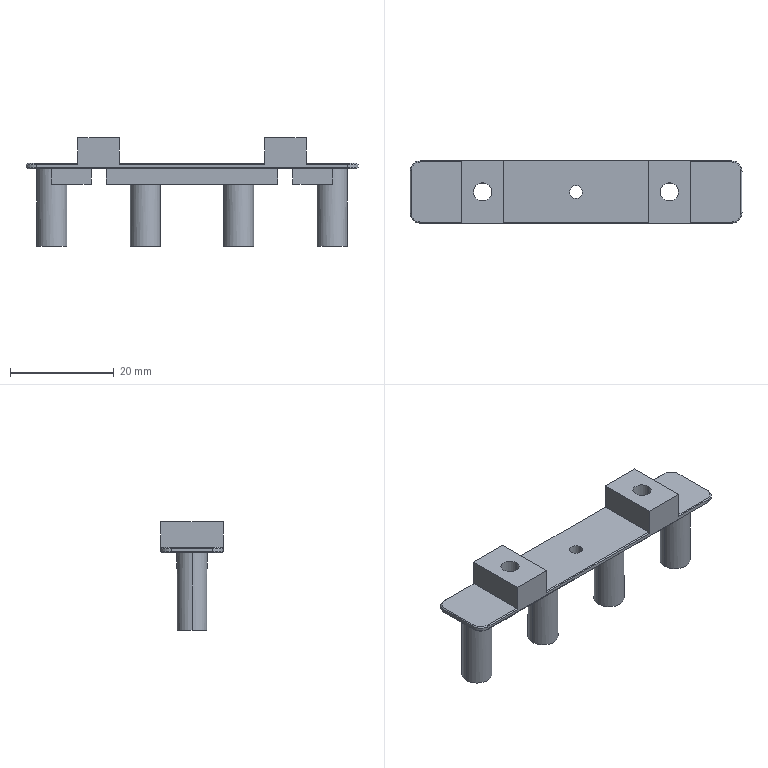NC program | NX | posted with a generic post | part box 64 x 12 x 21 mm
Lines 928 to 2253 of 2253:
(FLOOR_WALL_1_COPY_COPY , TOOL : D6)
N1848 T12 M6
N1850 G54
N1852 G17 G0 G90 X21.496 Y-7.4 S9500 M3
N1854 G43 Z30. H12
N1856 Z-10.5
N1858 G94 G1 Z-12. F1500.
N1860 Y-3.497
N1862 G3 X21.518 Y-2.897 R0.6
N1864 G1 X14.482
N1866 G3 X15.083 Y-1.199 R6.2
N1868 G1 X20.917
N1870 G2 X20.82 Y0.5 R6.2
N1872 G1 X15.18
N1874 G3 X14.797 Y2.198 R6.2
N1876 G1 X21.203
N1878 G2 X22.178 Y3.897 R6.2
N1880 G1 X13.822
N1882 G3 X11.67 Y5.595 R6.2
N1884 G1 X24.33
N1886 Z-10.5
N1888 G0 Z30.
N1890 X25.8 Y-7.302
N1892 Z-10.5
N1894 G1 Z-12.
N1896 X25.541 Y-6.048
N1898 G3 X25.143 Y-5.6 R0.6
N1900 G2 X25.143 Y5.6 R5.9
N1902 G3 X25.541 Y6.048 R0.6
N1904 G1 X25.8 Y7.302
N1906 Z-10.5
N1908 G0 X10.2
N1910 G1 Z-12.
N1912 X10.459 Y6.048
N1914 G3 X10.857 Y5.6 R0.6
N1916 G2 X10.857 Y-5.6 R5.9
N1918 G3 X10.459 Y-6.048 R0.6
N1920 G1 X10.2 Y-7.302
N1922 Z-10.5
N1924 G0 Z30.
N1926 X3.496 Y-7.4
N1928 Z-10.5
N1930 G1 Z-12.
N1932 Y-3.497
N1934 G3 X3.518 Y-2.897 R0.6
N1936 G1 X-3.518
N1938 G3 X-2.917 Y-1.199 R6.2
N1940 G1 X2.917
N1942 G2 X2.82 Y0.5 R6.2
N1944 G1 X-2.82
N1946 G3 X-3.203 Y2.198 R6.2
N1948 G1 X3.203
N1950 G2 X4.178 Y3.897 R6.2
N1952 G1 X-4.178
N1954 G3 X-6.33 Y5.595 R6.2
N1956 G1 X6.33
N1958 Z-10.5
N1960 G0 Z30.
N1962 X7.8 Y-7.302
N1964 Z-10.5
N1966 G1 Z-12.
N1968 X7.541 Y-6.048
N1970 G3 X7.143 Y-5.6 R0.6
N1972 G2 X7.143 Y5.6 R5.9
N1974 G3 X7.541 Y6.048 R0.6
N1976 G1 X7.8 Y7.302
N1978 Z-10.5
N1980 G0 X-7.8
N1982 G1 Z-12.
N1984 X-7.541 Y6.048
N1986 G3 X-7.143 Y5.6 R0.6
N1988 G2 X-7.143 Y-5.6 R5.9
N1990 G3 X-7.541 Y-6.048 R0.6
N1992 G1 X-7.8 Y-7.302
N1994 Z-10.5
N1996 G0 Z30.
N1998 X-14.504 Y-7.4
N2000 Z-10.5
N2002 G1 Z-12.
N2004 Y-3.497
N2006 G3 X-14.482 Y-2.897 R0.6
N2008 G1 X-21.518
N2010 G3 X-20.917 Y-1.199 R6.2
N2012 G1 X-15.083
N2014 G2 X-15.18 Y0.5 R6.2
N2016 G1 X-20.82
N2018 G3 X-21.203 Y2.198 R6.2
N2020 G1 X-14.797
N2022 G2 X-13.822 Y3.897 R6.2
N2024 G1 X-22.178
N2026 G3 X-24.33 Y5.595 R6.2
N2028 G1 X-11.67
N2030 Z-10.5
N2032 G0 Z30.
N2034 X-10.2 Y-7.302
N2036 Z-10.5
N2038 G1 Z-12.
N2040 X-10.459 Y-6.048
N2042 G3 X-10.857 Y-5.6 R0.6
N2044 G2 X-10.857 Y5.6 R5.9
N2046 G3 X-10.459 Y6.048 R0.6
N2048 G1 X-10.2 Y7.302
N2050 Z-10.5
N2052 G0 X-25.8
N2054 G1 Z-12.
N2056 X-25.541 Y6.048
N2058 G3 X-25.143 Y5.6 R0.6
N2060 G2 X-25.143 Y-5.6 R5.9
N2062 G3 X-25.541 Y-6.048 R0.6
N2064 G1 X-25.8 Y-7.302
N2066 Z-10.5
N2068 G0 Z30.
N2070 X35.548 Y-6.939
N2072 Z-13.5
N2074 G1 Z-15.
N2076 X35.011 Y-6.009
N2078 G3 X34.492 Y-5.709 R0.6
N2080 G1 X29.418
N2082 G3 X32.164 Y-3.432 R6.2
N2084 G1 X34.8
N2086 Y-1.154
N2088 X33.092
N2090 G3 X33.097 Y1.123 R6.2
N2092 G1 X34.8
N2094 Y3.4
N2096 X32.185
N2098 G3 X29.492 Y5.677 R6.2
N2100 G1 X34.508
N2102 G2 X35.027 Y5.377 R0.6
N2104 G1 X36.3 Y3.173
N2106 Z-13.5
N2108 G0 Z30.
N2110 X-29.057 Y-10.3
N2112 Z-13.5
N2114 G1 Z-15.
N2116 Y-6.188
N2118 G3 X-29.418 Y-5.709 R0.6
N2120 G1 X-34.492
N2122 X-34.601 Y-5.495
N2124 X-34.8 Y-4.236
N2126 Y-3.432
N2128 X-32.164
N2130 G2 X-33.092 Y-1.154 R6.2
N2132 G1 X-34.8
N2134 Y1.123
N2136 X-33.097
N2138 G2 X-32.185 Y3.4 R6.2
N2140 G1 X-34.8
N2142 Y4.236
N2144 X-34.601 Y5.495
N2146 X-34.508 Y5.677
N2148 X-29.492
N2150 Z-13.5
N2152 G0 Z30.
N2154 X34.253 Y8.625
N2156 Z-13.5
N2158 G1 Z-15.
N2160 X33.283 Y7.654
N2162 G3 X32.763 Y7.954 R0.6
N2164 G1 X-32.763
N2166 G3 X-33.283 Y7.654 R0.6
N2168 G1 X-31.058 Y4.716
N2170 G3 X-30.462 Y4.778 R0.6
N2172 G2 X-27. Y5.9 R5.9
N2174 G1 X27.
N2176 G2 X32.9 Y0. R5.9
N2178 X27. Y-5.9 R5.9
N2180 G1 X-27.
N2182 G2 X-30.462 Y4.778 R5.9
N2184 G3 X-30.217 Y5.326 R0.6
N2186 G1 X-30.382 Y6.918
N2188 Z-13.5
N2190 G0 Z30.
N2192 X18.11 Y0.224
N2194 Z-13.4
N2196 G1 X18. Y0.28 Z-13.433
N2198 X17.775 Y0.166 Z-13.501
N2200 X17.72 Y0. Z-13.548
N2202 X17.777 Y-0.113 Z-13.582
N2204 X17.814 Y-0.186 Z-13.604
N2206 X18. Y-0.28 Z-13.659
N2208 X18.113 Y-0.223 Z-13.693
N2210 X18.225 Y-0.166 Z-13.727
N2212 X18.28 Y0. Z-13.774
N2214 X18.223 Y0.113 Z-13.808
N2216 X18.186 Y0.186 Z-13.83
N2218 X18. Y0.28 Z-13.886
N2220 X17.775 Y0.166 Z-13.953
N2222 X17.72 Y0. Z-14.
N2224 X17.777 Y-0.113 Z-14.034
N2226 X17.814 Y-0.186 Z-14.056
N2228 X18. Y-0.28 Z-14.112
N2230 X18.113 Y-0.223 Z-14.146
N2232 X18.225 Y-0.166 Z-14.18
N2234 X18.28 Y0. Z-14.227
N2236 X18.223 Y0.113 Z-14.26
N2238 X18.186 Y0.186 Z-14.282
N2240 X18. Y0.28 Z-14.338
N2242 X17.775 Y0.166 Z-14.406
N2244 X17.72 Y0. Z-14.453
N2246 X17.777 Y-0.113 Z-14.487
N2248 X17.814 Y-0.186 Z-14.509
N2250 X18. Y-0.28 Z-14.564
N2252 X18.113 Y-0.223 Z-14.598
N2254 X18.225 Y-0.166 Z-14.632
N2256 X18.28 Y0. Z-14.679
N2258 X18.223 Y0.113 Z-14.713
N2260 X18.186 Y0.186 Z-14.735
N2262 X18. Y0.28 Z-14.791
N2264 X17.775 Y0.166 Z-14.858
N2266 X17.72 Y0. Z-14.905
N2268 X17.777 Y-0.113 Z-14.939
N2270 X17.814 Y-0.186 Z-14.961
N2272 X17.944 Y-0.252 Z-15.
N2274 X18. Y-0.28
N2276 X18.113 Y-0.223
N2278 G3 X18.113 Y0.223 R0.25
N2280 G1 X18. Y0.28
N2282 X17.887 Y0.223
N2284 G3 X17.887 Y-0.223 R0.25
N2286 G1 X17.944 Y-0.252
N2288 G3 X17.968 Y0.047 R0.3
N2290 G1 Z-13.5
N2292 G0 Z30.
N2294 X-17.89 Y0.224
N2296 Z-13.4
N2298 G1 X-18. Y0.28 Z-13.433
N2300 X-18.225 Y0.166 Z-13.501
N2302 X-18.28 Y0. Z-13.548
N2304 X-18.223 Y-0.113 Z-13.582
N2306 X-18.186 Y-0.186 Z-13.604
N2308 X-18. Y-0.28 Z-13.659
N2310 X-17.775 Y-0.166 Z-13.727
N2312 X-17.72 Y0. Z-13.774
N2314 X-17.777 Y0.113 Z-13.808
N2316 X-17.814 Y0.186 Z-13.83
N2318 X-18. Y0.28 Z-13.886
N2320 X-18.225 Y0.166 Z-13.953
N2322 X-18.28 Y0. Z-14.
N2324 X-18.223 Y-0.113 Z-14.034
N2326 X-18.186 Y-0.186 Z-14.056
N2328 X-18. Y-0.28 Z-14.112
N2330 X-17.775 Y-0.166 Z-14.18
N2332 X-17.72 Y0. Z-14.227
N2334 X-17.777 Y0.113 Z-14.26
N2336 X-17.814 Y0.186 Z-14.282
N2338 X-18. Y0.28 Z-14.338
N2340 X-18.225 Y0.166 Z-14.406
N2342 X-18.28 Y0. Z-14.453
N2344 X-18.223 Y-0.113 Z-14.487
N2346 X-18.186 Y-0.186 Z-14.509
N2348 X-18. Y-0.28 Z-14.564
N2350 X-17.775 Y-0.166 Z-14.632
N2352 X-17.72 Y0. Z-14.679
N2354 X-17.777 Y0.113 Z-14.713
N2356 X-17.814 Y0.186 Z-14.735
N2358 X-18. Y0.28 Z-14.791
N2360 X-18.225 Y0.166 Z-14.858
N2362 X-18.28 Y0. Z-14.905
N2364 X-18.223 Y-0.113 Z-14.939
N2366 X-18.186 Y-0.186 Z-14.961
N2368 X-18.056 Y-0.252 Z-15.
N2370 X-18. Y-0.28
N2372 X-17.887 Y-0.223
N2374 G3 X-17.887 Y0.223 R0.25
N2376 G1 X-18. Y0.28
N2378 X-18.113 Y0.223
N2380 G3 X-18.113 Y-0.223 R0.25
N2382 G1 X-18.056 Y-0.252
N2384 G3 X-18.032 Y0.047 R0.3
N2386 G1 Z-13.5
N2388 G0 Z30.
(ZLEVEL_PROFILE_COPY , TOOL : D6)
N2390 X-26.002 Y-7.029
N2392 Z-3.
N2394 G1 Z-4. F1000.
N2396 X-26.48 Y-6.2
N2398 G3 X-27. Y-5.9 R0.6
N2400 G1 X-27.045 F1200.
N2402 G2 X-32.9 Y0.045 R5.9
N2404 X-27. Y-5.9 R-5.9
N2406 G1 X-27.299 Y-5.892 Z-4.032
N2408 X-27.597 Y-5.87 Z-4.065
N2410 X-27.893 Y-5.832 Z-4.097
N2412 X-28.188 Y-5.779 Z-4.129
N2414 X-28.479 Y-5.712 Z-4.161
N2416 X-28.766 Y-5.629 Z-4.194
N2418 X-29.049 Y-5.533 Z-4.226
N2420 X-29.327 Y-5.422 Z-4.258
N2422 X-29.598 Y-5.297 Z-4.29
N2424 X-29.863 Y-5.159 Z-4.323
N2426 X-30.121 Y-5.007 Z-4.355
N2428 X-30.37 Y-4.843 Z-4.387
N2430 X-30.611 Y-4.666 Z-4.419
N2432 X-30.843 Y-4.477 Z-4.452
N2434 X-31.065 Y-4.276 Z-4.484
N2436 X-31.276 Y-4.065 Z-4.516
N2438 X-31.477 Y-3.843 Z-4.548
N2440 X-31.666 Y-3.611 Z-4.581
N2442 X-31.843 Y-3.37 Z-4.613
N2444 X-32.007 Y-3.121 Z-4.645
N2446 X-32.159 Y-2.863 Z-4.677
N2448 X-32.297 Y-2.598 Z-4.71
N2450 X-32.422 Y-2.327 Z-4.742
N2452 X-32.533 Y-2.049 Z-4.774
N2454 X-32.629 Y-1.766 Z-4.806
N2456 X-32.712 Y-1.479 Z-4.839
N2458 X-32.779 Y-1.188 Z-4.871
N2460 X-32.832 Y-0.893 Z-4.903
N2462 X-32.87 Y-0.597 Z-4.935
N2464 X-32.892 Y-0.299 Z-4.968
N2466 X-32.9 Y0. Z-5.
N2468 X-32.892 Y0.299 Z-5.032
N2470 X-32.87 Y0.597 Z-5.065
N2472 X-32.832 Y0.893 Z-5.097
N2474 X-32.779 Y1.188 Z-5.129
N2476 X-32.712 Y1.479 Z-5.161
N2478 X-32.629 Y1.766 Z-5.194
N2480 X-32.533 Y2.049 Z-5.226
N2482 X-32.422 Y2.327 Z-5.258
N2484 X-32.297 Y2.598 Z-5.29
N2486 X-32.159 Y2.863 Z-5.323
N2488 X-32.007 Y3.121 Z-5.355
N2490 X-31.843 Y3.37 Z-5.387
N2492 X-31.666 Y3.611 Z-5.419
N2494 X-31.477 Y3.843 Z-5.452
N2496 X-31.276 Y4.065 Z-5.484
N2498 X-31.065 Y4.276 Z-5.516
N2500 X-30.843 Y4.477 Z-5.548
N2502 X-30.611 Y4.666 Z-5.581
N2504 X-30.37 Y4.843 Z-5.613
N2506 X-30.121 Y5.007 Z-5.645
N2508 X-29.863 Y5.159 Z-5.677
N2510 X-29.598 Y5.297 Z-5.71
N2512 X-29.327 Y5.422 Z-5.742
N2514 X-29.049 Y5.533 Z-5.774
N2516 X-28.766 Y5.629 Z-5.806
N2518 X-28.479 Y5.712 Z-5.839
N2520 X-28.188 Y5.779 Z-5.871
N2522 X-27.893 Y5.832 Z-5.903
N2524 X-27.597 Y5.87 Z-5.935
N2526 X-27.299 Y5.892 Z-5.968
N2528 X-27. Y5.9 Z-6.
N2530 X-26.701 Y5.892 Z-6.032
N2532 X-26.403 Y5.87 Z-6.065
N2534 X-26.107 Y5.832 Z-6.097
N2536 X-25.812 Y5.779 Z-6.129
N2538 X-25.521 Y5.712 Z-6.161
N2540 X-25.234 Y5.629 Z-6.194
N2542 X-24.951 Y5.533 Z-6.226
N2544 X-24.673 Y5.422 Z-6.258
N2546 X-24.402 Y5.297 Z-6.29
N2548 X-24.137 Y5.159 Z-6.323
N2550 X-23.879 Y5.007 Z-6.355
N2552 X-23.63 Y4.843 Z-6.387
N2554 X-23.389 Y4.666 Z-6.419
N2556 X-23.157 Y4.477 Z-6.452
N2558 X-22.935 Y4.276 Z-6.484
N2560 X-22.724 Y4.065 Z-6.516
N2562 X-22.523 Y3.843 Z-6.548
N2564 X-22.334 Y3.611 Z-6.581
N2566 X-22.157 Y3.37 Z-6.613
N2568 X-21.993 Y3.121 Z-6.645
N2570 X-21.841 Y2.863 Z-6.677
N2572 X-21.703 Y2.598 Z-6.71
N2574 X-21.578 Y2.327 Z-6.742
N2576 X-21.467 Y2.049 Z-6.774
N2578 X-21.371 Y1.766 Z-6.806
N2580 X-21.288 Y1.479 Z-6.839
N2582 X-21.221 Y1.188 Z-6.871
N2584 X-21.168 Y0.893 Z-6.903
N2586 X-21.13 Y0.597 Z-6.935
N2588 X-21.108 Y0.299 Z-6.968
N2590 X-21.1 Y0. Z-7.
N2592 X-21.108 Y-0.299 Z-7.032
N2594 X-21.13 Y-0.597 Z-7.065
N2596 X-21.168 Y-0.893 Z-7.097
N2598 X-21.221 Y-1.188 Z-7.129
N2600 X-21.288 Y-1.479 Z-7.161
N2602 X-21.371 Y-1.766 Z-7.194
N2604 X-21.467 Y-2.049 Z-7.226
N2606 X-21.578 Y-2.327 Z-7.258
N2608 X-21.703 Y-2.598 Z-7.29
N2610 X-21.841 Y-2.863 Z-7.323
N2612 X-21.993 Y-3.121 Z-7.355
N2614 X-22.157 Y-3.37 Z-7.387
N2616 X-22.334 Y-3.611 Z-7.419
N2618 X-22.523 Y-3.843 Z-7.452
N2620 X-22.724 Y-4.065 Z-7.484
N2622 X-22.935 Y-4.276 Z-7.516
N2624 X-23.157 Y-4.477 Z-7.548
N2626 X-23.389 Y-4.666 Z-7.581
N2628 X-23.63 Y-4.843 Z-7.613
N2630 X-23.879 Y-5.007 Z-7.645
N2632 X-24.137 Y-5.159 Z-7.677
N2634 X-24.402 Y-5.297 Z-7.71
N2636 X-24.673 Y-5.422 Z-7.742
N2638 X-24.951 Y-5.533 Z-7.774
N2640 X-25.234 Y-5.629 Z-7.806
N2642 X-25.521 Y-5.712 Z-7.839
N2644 X-25.812 Y-5.779 Z-7.871
N2646 X-26.107 Y-5.832 Z-7.903
N2648 X-26.403 Y-5.87 Z-7.935
N2650 X-26.701 Y-5.892 Z-7.968
N2652 X-27. Y-5.9 Z-8.
N2654 X-27.299 Y-5.892 Z-8.032
N2656 X-27.597 Y-5.87 Z-8.065
N2658 X-27.893 Y-5.832 Z-8.097
N2660 X-28.188 Y-5.779 Z-8.129
N2662 X-28.479 Y-5.712 Z-8.161
N2664 X-28.766 Y-5.629 Z-8.194
N2666 X-29.049 Y-5.533 Z-8.226
N2668 X-29.327 Y-5.422 Z-8.258
N2670 X-29.598 Y-5.297 Z-8.29
N2672 X-29.863 Y-5.159 Z-8.323
N2674 X-30.121 Y-5.007 Z-8.355
N2676 X-30.37 Y-4.843 Z-8.387
N2678 X-30.611 Y-4.666 Z-8.419
N2680 X-30.843 Y-4.477 Z-8.452
N2682 X-31.065 Y-4.276 Z-8.484
N2684 X-31.276 Y-4.065 Z-8.516
N2686 X-31.477 Y-3.843 Z-8.548
N2688 X-31.666 Y-3.611 Z-8.581
N2690 X-31.843 Y-3.37 Z-8.613
N2692 X-32.007 Y-3.121 Z-8.645
N2694 X-32.159 Y-2.863 Z-8.677
N2696 X-32.297 Y-2.598 Z-8.71
N2698 X-32.422 Y-2.327 Z-8.742
N2700 X-32.533 Y-2.049 Z-8.774
N2702 X-32.629 Y-1.766 Z-8.806
N2704 X-32.712 Y-1.479 Z-8.839
N2706 X-32.779 Y-1.188 Z-8.871
N2708 X-32.832 Y-0.893 Z-8.903
N2710 X-32.87 Y-0.597 Z-8.935
N2712 X-32.892 Y-0.299 Z-8.968
N2714 X-32.9 Y0. Z-9.
N2716 X-32.892 Y0.299 Z-9.032
N2718 X-32.87 Y0.597 Z-9.065
N2720 X-32.832 Y0.893 Z-9.097
N2722 X-32.779 Y1.188 Z-9.129
N2724 X-32.712 Y1.479 Z-9.161
N2726 X-32.629 Y1.766 Z-9.194
N2728 X-32.533 Y2.049 Z-9.226
N2730 X-32.422 Y2.327 Z-9.258
N2732 X-32.297 Y2.598 Z-9.29
N2734 X-32.159 Y2.863 Z-9.323
N2736 X-32.007 Y3.121 Z-9.355
N2738 X-31.843 Y3.37 Z-9.387
N2740 X-31.666 Y3.611 Z-9.419
N2742 X-31.477 Y3.843 Z-9.452
N2744 X-31.276 Y4.065 Z-9.484
N2746 X-31.065 Y4.276 Z-9.516
N2748 X-30.843 Y4.477 Z-9.548
N2750 X-30.611 Y4.666 Z-9.581
N2752 X-30.37 Y4.843 Z-9.613
N2754 X-30.121 Y5.007 Z-9.645
N2756 X-29.863 Y5.159 Z-9.677
N2758 X-29.598 Y5.297 Z-9.71
N2760 X-29.327 Y5.422 Z-9.742
N2762 X-29.049 Y5.533 Z-9.774
N2764 X-28.766 Y5.629 Z-9.806
N2766 X-28.479 Y5.712 Z-9.839
N2768 X-28.188 Y5.779 Z-9.871
N2770 X-27.893 Y5.832 Z-9.903
N2772 X-27.597 Y5.87 Z-9.935
N2774 X-27.299 Y5.892 Z-9.968
N2776 X-27. Y5.9 Z-10.
N2778 X-26.701 Y5.892 Z-10.032
N2780 X-26.403 Y5.87 Z-10.065
N2782 X-26.107 Y5.832 Z-10.097
N2784 X-25.812 Y5.779 Z-10.129
N2786 X-25.521 Y5.712 Z-10.161
N2788 X-25.234 Y5.629 Z-10.194
N2790 X-24.951 Y5.533 Z-10.226
N2792 X-24.673 Y5.422 Z-10.258
N2794 X-24.402 Y5.297 Z-10.29
N2796 X-24.137 Y5.159 Z-10.323
N2798 X-23.879 Y5.007 Z-10.355
N2800 X-23.63 Y4.843 Z-10.387
N2802 X-23.389 Y4.666 Z-10.419
N2804 X-23.157 Y4.477 Z-10.452
N2806 X-22.935 Y4.276 Z-10.484
N2808 X-22.724 Y4.065 Z-10.516
N2810 X-22.523 Y3.843 Z-10.548
N2812 X-22.334 Y3.611 Z-10.581
N2814 X-22.157 Y3.37 Z-10.613
N2816 X-21.993 Y3.121 Z-10.645
N2818 X-21.841 Y2.863 Z-10.677
N2820 X-21.703 Y2.598 Z-10.71
N2822 X-21.578 Y2.327 Z-10.742
N2824 X-21.467 Y2.049 Z-10.774
N2826 X-21.371 Y1.766 Z-10.806
N2828 X-21.288 Y1.479 Z-10.839
N2830 X-21.221 Y1.188 Z-10.871
N2832 X-21.168 Y0.893 Z-10.903
N2834 X-21.13 Y0.597 Z-10.935
N2836 X-21.108 Y0.299 Z-10.968
N2838 X-21.1 Y0. Z-11.
N2840 X-21.108 Y-0.299 Z-11.032
N2842 X-21.13 Y-0.597 Z-11.065
N2844 X-21.168 Y-0.893 Z-11.097
N2846 X-21.221 Y-1.188 Z-11.129
N2848 X-21.288 Y-1.479 Z-11.161
N2850 X-21.371 Y-1.766 Z-11.194
N2852 X-21.467 Y-2.049 Z-11.226
N2854 X-21.578 Y-2.327 Z-11.258
N2856 X-21.703 Y-2.598 Z-11.29
N2858 X-21.841 Y-2.863 Z-11.323
N2860 X-21.993 Y-3.121 Z-11.355
N2862 X-22.157 Y-3.37 Z-11.387
N2864 X-22.334 Y-3.611 Z-11.419
N2866 X-22.523 Y-3.843 Z-11.452
N2868 X-22.724 Y-4.065 Z-11.484
N2870 X-22.935 Y-4.276 Z-11.516
N2872 X-23.157 Y-4.477 Z-11.548
N2874 X-23.389 Y-4.666 Z-11.581
N2876 X-23.63 Y-4.843 Z-11.613
N2878 X-23.879 Y-5.007 Z-11.645
N2880 X-24.137 Y-5.159 Z-11.677
N2882 X-24.402 Y-5.297 Z-11.71
N2884 X-24.673 Y-5.422 Z-11.742
N2886 X-24.951 Y-5.533 Z-11.774
N2888 X-25.234 Y-5.629 Z-11.806
N2890 X-25.521 Y-5.712 Z-11.839
N2892 X-25.812 Y-5.779 Z-11.871
N2894 X-26.107 Y-5.832 Z-11.903
N2896 X-26.403 Y-5.87 Z-11.935
N2898 X-26.701 Y-5.892 Z-11.968
N2900 X-27. Y-5.9 Z-12.
N2902 X-27.045
N2904 G2 X-32.9 Y0.045 R5.9
N2906 X-27. Y-5.9 R-5.9
N2908 G3 X-27.52 Y-6.2 R0.6
N2910 G1 X-27.998 Y-7.029
N2912 Z-11.
N2914 G0 Z30.
N2916 X-8.002
N2918 Z-3.
N2920 G1 Z-4. F1000.
N2922 X-8.48 Y-6.2
N2924 G3 X-9. Y-5.9 R0.6
N2926 G2 X-14.9 Y0. R5.9 F1200.
N2928 X-9. Y-5.9 R-5.9
N2930 G1 X-9.299 Y-5.892 Z-4.032
N2932 X-9.597 Y-5.87 Z-4.065
N2934 X-9.893 Y-5.832 Z-4.097
N2936 X-10.188 Y-5.779 Z-4.129
N2938 X-10.479 Y-5.712 Z-4.161
N2940 X-10.766 Y-5.629 Z-4.194
N2942 X-11.049 Y-5.533 Z-4.226
N2944 X-11.327 Y-5.422 Z-4.258
N2946 X-11.598 Y-5.297 Z-4.29
N2948 X-11.863 Y-5.159 Z-4.323
N2950 X-12.121 Y-5.007 Z-4.355
N2952 X-12.37 Y-4.843 Z-4.387
N2954 X-12.611 Y-4.666 Z-4.419
N2956 X-12.843 Y-4.477 Z-4.452
N2958 X-13.065 Y-4.276 Z-4.484
N2960 X-13.276 Y-4.065 Z-4.516
N2962 X-13.477 Y-3.843 Z-4.548
N2964 X-13.666 Y-3.611 Z-4.581
N2966 X-13.843 Y-3.37 Z-4.613
N2968 X-14.007 Y-3.121 Z-4.645
N2970 X-14.159 Y-2.863 Z-4.677
N2972 X-14.297 Y-2.598 Z-4.71
N2974 X-14.422 Y-2.327 Z-4.742
N2976 X-14.533 Y-2.049 Z-4.774
N2978 X-14.629 Y-1.766 Z-4.806
N2980 X-14.712 Y-1.479 Z-4.839
N2982 X-14.779 Y-1.188 Z-4.871
N2984 X-14.832 Y-0.893 Z-4.903
N2986 X-14.87 Y-0.597 Z-4.935
N2988 X-14.892 Y-0.299 Z-4.968
N2990 X-14.9 Y0. Z-5.
N2992 X-14.892 Y0.299 Z-5.032
N2994 X-14.87 Y0.597 Z-5.065
N2996 X-14.832 Y0.893 Z-5.097
N2998 X-14.779 Y1.188 Z-5.129
N3000 X-14.712 Y1.479 Z-5.161
N3002 X-14.629 Y1.766 Z-5.194
N3004 X-14.533 Y2.049 Z-5.226
N3006 X-14.422 Y2.327 Z-5.258
N3008 X-14.297 Y2.598 Z-5.29
N3010 X-14.159 Y2.863 Z-5.323
N3012 X-14.007 Y3.121 Z-5.355
N3014 X-13.843 Y3.37 Z-5.387
N3016 X-13.666 Y3.611 Z-5.419
N3018 X-13.477 Y3.843 Z-5.452
N3020 X-13.276 Y4.065 Z-5.484
N3022 X-13.065 Y4.276 Z-5.516
N3024 X-12.843 Y4.477 Z-5.548
N3026 X-12.611 Y4.666 Z-5.581
N3028 X-12.37 Y4.843 Z-5.613
N3030 X-12.121 Y5.007 Z-5.645
N3032 X-11.863 Y5.159 Z-5.677
N3034 X-11.598 Y5.297 Z-5.71
N3036 X-11.327 Y5.422 Z-5.742
N3038 X-11.049 Y5.533 Z-5.774
N3040 X-10.766 Y5.629 Z-5.806
N3042 X-10.479 Y5.712 Z-5.839
N3044 X-10.188 Y5.779 Z-5.871
N3046 X-9.893 Y5.832 Z-5.903
N3048 X-9.597 Y5.87 Z-5.935
N3050 X-9.299 Y5.892 Z-5.968
N3052 X-9. Y5.9 Z-6.
N3054 X-8.701 Y5.892 Z-6.032
N3056 X-8.403 Y5.87 Z-6.065
N3058 X-8.107 Y5.832 Z-6.097
N3060 X-7.812 Y5.779 Z-6.129
N3062 X-7.521 Y5.712 Z-6.161
N3064 X-7.234 Y5.629 Z-6.194
N3066 X-6.951 Y5.533 Z-6.226
N3068 X-6.673 Y5.422 Z-6.258
N3070 X-6.402 Y5.297 Z-6.29
N3072 X-6.137 Y5.159 Z-6.323
N3074 X-5.879 Y5.007 Z-6.355
N3076 X-5.63 Y4.843 Z-6.387
N3078 X-5.389 Y4.666 Z-6.419
N3080 X-5.157 Y4.477 Z-6.452
N3082 X-4.935 Y4.276 Z-6.484
N3084 X-4.724 Y4.065 Z-6.516
N3086 X-4.523 Y3.843 Z-6.548
N3088 X-4.334 Y3.611 Z-6.581
N3090 X-4.157 Y3.37 Z-6.613
N3092 X-3.993 Y3.121 Z-6.645
N3094 X-3.841 Y2.863 Z-6.677
N3096 X-3.703 Y2.598 Z-6.71
N3098 X-3.578 Y2.327 Z-6.742
N3100 X-3.467 Y2.049 Z-6.774
N3102 X-3.371 Y1.766 Z-6.806
N3104 X-3.288 Y1.479 Z-6.839
N3106 X-3.221 Y1.188 Z-6.871
N3108 X-3.168 Y0.893 Z-6.903
N3110 X-3.13 Y0.597 Z-6.935
N3112 X-3.108 Y0.299 Z-6.968
N3114 X-3.1 Y0. Z-7.
N3116 X-3.108 Y-0.299 Z-7.032
N3118 X-3.13 Y-0.597 Z-7.065
N3120 X-3.168 Y-0.893 Z-7.097
N3122 X-3.221 Y-1.188 Z-7.129
N3124 X-3.288 Y-1.479 Z-7.161
N3126 X-3.371 Y-1.766 Z-7.194
N3128 X-3.467 Y-2.049 Z-7.226
N3130 X-3.578 Y-2.327 Z-7.258
N3132 X-3.703 Y-2.598 Z-7.29
N3134 X-3.841 Y-2.863 Z-7.323
N3136 X-3.993 Y-3.121 Z-7.355
N3138 X-4.157 Y-3.37 Z-7.387
N3140 X-4.334 Y-3.611 Z-7.419
N3142 X-4.523 Y-3.843 Z-7.452
N3144 X-4.724 Y-4.065 Z-7.484
N3146 X-4.935 Y-4.276 Z-7.516
N3148 X-5.157 Y-4.477 Z-7.548
N3150 X-5.389 Y-4.666 Z-7.581
N3152 X-5.63 Y-4.843 Z-7.613
N3154 X-5.879 Y-5.007 Z-7.645
N3156 X-6.137 Y-5.159 Z-7.677
N3158 X-6.402 Y-5.297 Z-7.71
N3160 X-6.673 Y-5.422 Z-7.742
N3162 X-6.951 Y-5.533 Z-7.774
N3164 X-7.234 Y-5.629 Z-7.806
N3166 X-7.521 Y-5.712 Z-7.839
N3168 X-7.812 Y-5.779 Z-7.871
N3170 X-8.107 Y-5.832 Z-7.903
N3172 X-8.403 Y-5.87 Z-7.935
N3174 X-8.701 Y-5.892 Z-7.968
N3176 X-9. Y-5.9 Z-8.
N3178 X-9.299 Y-5.892 Z-8.032
N3180 X-9.597 Y-5.87 Z-8.065
N3182 X-9.893 Y-5.832 Z-8.097
N3184 X-10.188 Y-5.779 Z-8.129
N3186 X-10.479 Y-5.712 Z-8.161
N3188 X-10.766 Y-5.629 Z-8.194
N3190 X-11.049 Y-5.533 Z-8.226
N3192 X-11.327 Y-5.422 Z-8.258
N3194 X-11.598 Y-5.297 Z-8.29
N3196 X-11.863 Y-5.159 Z-8.323
N3198 X-12.121 Y-5.007 Z-8.355
N3200 X-12.37 Y-4.843 Z-8.387
N3202 X-12.611 Y-4.666 Z-8.419
N3204 X-12.843 Y-4.477 Z-8.452
N3206 X-13.065 Y-4.276 Z-8.484
N3208 X-13.276 Y-4.065 Z-8.516
N3210 X-13.477 Y-3.843 Z-8.548
N3212 X-13.666 Y-3.611 Z-8.581
N3214 X-13.843 Y-3.37 Z-8.613
N3216 X-14.007 Y-3.121 Z-8.645
N3218 X-14.159 Y-2.863 Z-8.677
N3220 X-14.297 Y-2.598 Z-8.71
N3222 X-14.422 Y-2.327 Z-8.742
N3224 X-14.533 Y-2.049 Z-8.774
N3226 X-14.629 Y-1.766 Z-8.806
N3228 X-14.712 Y-1.479 Z-8.839
N3230 X-14.779 Y-1.188 Z-8.871
N3232 X-14.832 Y-0.893 Z-8.903
N3234 X-14.87 Y-0.597 Z-8.935
N3236 X-14.892 Y-0.299 Z-8.968
N3238 X-14.9 Y0. Z-9.
N3240 X-14.892 Y0.299 Z-9.032
N3242 X-14.87 Y0.597 Z-9.065
N3244 X-14.832 Y0.893 Z-9.097
N3246 X-14.779 Y1.188 Z-9.129
N3248 X-14.712 Y1.479 Z-9.161
N3250 X-14.629 Y1.766 Z-9.194
N3252 X-14.533 Y2.049 Z-9.226
N3254 X-14.422 Y2.327 Z-9.258
N3256 X-14.297 Y2.598 Z-9.29
N3258 X-14.159 Y2.863 Z-9.323
N3260 X-14.007 Y3.121 Z-9.355
N3262 X-13.843 Y3.37 Z-9.387
N3264 X-13.666 Y3.611 Z-9.419
N3266 X-13.477 Y3.843 Z-9.452
N3268 X-13.276 Y4.065 Z-9.484
N3270 X-13.065 Y4.276 Z-9.516
N3272 X-12.843 Y4.477 Z-9.548
N3274 X-12.611 Y4.666 Z-9.581
N3276 X-12.37 Y4.843 Z-9.613
N3278 X-12.121 Y5.007 Z-9.645
N3280 X-11.863 Y5.159 Z-9.677
N3282 X-11.598 Y5.297 Z-9.71
N3284 X-11.327 Y5.422 Z-9.742
N3286 X-11.049 Y5.533 Z-9.774
N3288 X-10.766 Y5.629 Z-9.806
N3290 X-10.479 Y5.712 Z-9.839
N3292 X-10.188 Y5.779 Z-9.871
N3294 X-9.893 Y5.832 Z-9.903
N3296 X-9.597 Y5.87 Z-9.935
N3298 X-9.299 Y5.892 Z-9.968
N3300 X-9. Y5.9 Z-10.
N3302 X-8.701 Y5.892 Z-10.032
N3304 X-8.403 Y5.87 Z-10.065
N3306 X-8.107 Y5.832 Z-10.097
N3308 X-7.812 Y5.779 Z-10.129
N3310 X-7.521 Y5.712 Z-10.161
N3312 X-7.234 Y5.629 Z-10.194
N3314 X-6.951 Y5.533 Z-10.226
N3316 X-6.673 Y5.422 Z-10.258
N3318 X-6.402 Y5.297 Z-10.29
N3320 X-6.137 Y5.159 Z-10.323
N3322 X-5.879 Y5.007 Z-10.355
N3324 X-5.63 Y4.843 Z-10.387
N3326 X-5.389 Y4.666 Z-10.419
N3328 X-5.157 Y4.477 Z-10.452
N3330 X-4.935 Y4.276 Z-10.484
N3332 X-4.724 Y4.065 Z-10.516
N3334 X-4.523 Y3.843 Z-10.548
N3336 X-4.334 Y3.611 Z-10.581
N3338 X-4.157 Y3.37 Z-10.613
N3340 X-3.993 Y3.121 Z-10.645
N3342 X-3.841 Y2.863 Z-10.677
N3344 X-3.703 Y2.598 Z-10.71
N3346 X-3.578 Y2.327 Z-10.742
N3348 X-3.467 Y2.049 Z-10.774
N3350 X-3.371 Y1.766 Z-10.806
N3352 X-3.288 Y1.479 Z-10.839
N3354 X-3.221 Y1.188 Z-10.871
N3356 X-3.168 Y0.893 Z-10.903
N3358 X-3.13 Y0.597 Z-10.935
N3360 X-3.108 Y0.299 Z-10.968
N3362 X-3.1 Y0. Z-11.
N3364 X-3.108 Y-0.299 Z-11.032
N3366 X-3.13 Y-0.597 Z-11.065
N3368 X-3.168 Y-0.893 Z-11.097
N3370 X-3.221 Y-1.188 Z-11.129
N3372 X-3.288 Y-1.479 Z-11.161
N3374 X-3.371 Y-1.766 Z-11.194
N3376 X-3.467 Y-2.049 Z-11.226
N3378 X-3.578 Y-2.327 Z-11.258
N3380 X-3.703 Y-2.598 Z-11.29
N3382 X-3.841 Y-2.863 Z-11.323
N3384 X-3.993 Y-3.121 Z-11.355
N3386 X-4.157 Y-3.37 Z-11.387
N3388 X-4.334 Y-3.611 Z-11.419
N3390 X-4.523 Y-3.843 Z-11.452
N3392 X-4.724 Y-4.065 Z-11.484
N3394 X-4.935 Y-4.276 Z-11.516
N3396 X-5.157 Y-4.477 Z-11.548
N3398 X-5.389 Y-4.666 Z-11.581
N3400 X-5.63 Y-4.843 Z-11.613
N3402 X-5.879 Y-5.007 Z-11.645
N3404 X-6.137 Y-5.159 Z-11.677
N3406 X-6.402 Y-5.297 Z-11.71
N3408 X-6.673 Y-5.422 Z-11.742
N3410 X-6.951 Y-5.533 Z-11.774
N3412 X-7.234 Y-5.629 Z-11.806
N3414 X-7.521 Y-5.712 Z-11.839
N3416 X-7.812 Y-5.779 Z-11.871
N3418 X-8.107 Y-5.832 Z-11.903
N3420 X-8.403 Y-5.87 Z-11.935
N3422 X-8.701 Y-5.892 Z-11.968
N3424 X-9. Y-5.9 Z-12.
N3426 G2 X-14.9 Y0. R5.9
N3428 X-9. Y-5.9 R-5.9
N3430 G3 X-9.52 Y-6.2 R0.6
N3432 G1 X-9.998 Y-7.029
N3434 Z-11.
N3436 G0 Z30.
N3438 X27.998
N3440 Z-3.
N3442 G1 Z-4. F1000.
N3444 X27.52 Y-6.2
N3446 G3 X27. Y-5.9 R0.6
N3448 G1 X26.924 F1200.
N3450 G2 X27. Y-5.9 R-5.9
N3452 G1 X26.701 Y-5.892 Z-4.032
N3454 X26.403 Y-5.87 Z-4.065
N3456 X26.107 Y-5.832 Z-4.097
N3458 X25.812 Y-5.779 Z-4.129
N3460 X25.521 Y-5.712 Z-4.161
N3462 X25.234 Y-5.629 Z-4.194
N3464 X24.951 Y-5.533 Z-4.226
N3466 X24.673 Y-5.422 Z-4.258
N3468 X24.402 Y-5.297 Z-4.29
N3470 X24.137 Y-5.159 Z-4.323
N3472 X23.879 Y-5.007 Z-4.355
N3474 X23.63 Y-4.843 Z-4.387
N3476 X23.389 Y-4.666 Z-4.419
N3478 X23.157 Y-4.477 Z-4.452
N3480 X22.935 Y-4.276 Z-4.484
N3482 X22.724 Y-4.065 Z-4.516
N3484 X22.523 Y-3.843 Z-4.548
N3486 X22.334 Y-3.611 Z-4.581
N3488 X22.157 Y-3.37 Z-4.613
N3490 X21.993 Y-3.121 Z-4.645
N3492 X21.841 Y-2.863 Z-4.677
N3494 X21.703 Y-2.598 Z-4.71
N3496 X21.578 Y-2.327 Z-4.742
N3498 X21.467 Y-2.049 Z-4.774
N3500 X21.371 Y-1.766 Z-4.806
N3502 X21.288 Y-1.479 Z-4.839
N3504 X21.221 Y-1.188 Z-4.871
N3506 X21.168 Y-0.893 Z-4.903
N3508 X21.13 Y-0.597 Z-4.935
N3510 X21.108 Y-0.299 Z-4.968
N3512 X21.1 Y0. Z-5.
N3514 X21.108 Y0.299 Z-5.032
N3516 X21.13 Y0.597 Z-5.065
N3518 X21.168 Y0.893 Z-5.097
N3520 X21.221 Y1.188 Z-5.129
N3522 X21.288 Y1.479 Z-5.161
N3524 X21.371 Y1.766 Z-5.194
N3526 X21.467 Y2.049 Z-5.226
N3528 X21.578 Y2.327 Z-5.258
N3530 X21.703 Y2.598 Z-5.29
N3532 X21.841 Y2.863 Z-5.323
N3534 X21.993 Y3.121 Z-5.355
N3536 X22.157 Y3.37 Z-5.387
N3538 X22.334 Y3.611 Z-5.419
N3540 X22.523 Y3.843 Z-5.452
N3542 X22.724 Y4.065 Z-5.484
N3544 X22.935 Y4.276 Z-5.516
N3546 X23.157 Y4.477 Z-5.548
N3548 X23.389 Y4.666 Z-5.581
N3550 X23.63 Y4.843 Z-5.613
N3552 X23.879 Y5.007 Z-5.645
N3554 X24.137 Y5.159 Z-5.677
N3556 X24.402 Y5.297 Z-5.71
N3558 X24.673 Y5.422 Z-5.742
N3560 X24.951 Y5.533 Z-5.774
N3562 X25.234 Y5.629 Z-5.806
N3564 X25.521 Y5.712 Z-5.839
N3566 X25.812 Y5.779 Z-5.871
N3568 X26.107 Y5.832 Z-5.903
N3570 X26.403 Y5.87 Z-5.935
N3572 X26.701 Y5.892 Z-5.968
N3574 X27. Y5.9 Z-6.
N3576 X27.299 Y5.892 Z-6.032
N3578 X27.597 Y5.87 Z-6.065
N3580 X27.893 Y5.832 Z-6.097
N3582 X28.188 Y5.779 Z-6.129
N3584 X28.479 Y5.712 Z-6.161
N3586 X28.766 Y5.629 Z-6.194
N3588 X29.049 Y5.533 Z-6.226
N3590 X29.327 Y5.422 Z-6.258
N3592 X29.598 Y5.297 Z-6.29
N3594 X29.863 Y5.159 Z-6.323
N3596 X30.121 Y5.007 Z-6.355
N3598 X30.37 Y4.843 Z-6.387
N3600 X30.611 Y4.666 Z-6.419
N3602 X30.843 Y4.477 Z-6.452
N3604 X31.065 Y4.276 Z-6.484
N3606 X31.276 Y4.065 Z-6.516
N3608 X31.477 Y3.843 Z-6.548
N3610 X31.666 Y3.611 Z-6.581
N3612 X31.843 Y3.37 Z-6.613
N3614 X32.007 Y3.121 Z-6.645
N3616 X32.159 Y2.863 Z-6.677
N3618 X32.297 Y2.598 Z-6.71
N3620 X32.422 Y2.327 Z-6.742
N3622 X32.533 Y2.049 Z-6.774
N3624 X32.629 Y1.766 Z-6.806
N3626 X32.712 Y1.479 Z-6.839
N3628 X32.779 Y1.188 Z-6.871
N3630 X32.832 Y0.893 Z-6.903
N3632 X32.87 Y0.597 Z-6.935
N3634 X32.892 Y0.299 Z-6.968
N3636 X32.9 Y0. Z-7.
N3638 X32.892 Y-0.299 Z-7.032
N3640 X32.87 Y-0.597 Z-7.065
N3642 X32.832 Y-0.893 Z-7.097
N3644 X32.779 Y-1.188 Z-7.129
N3646 X32.712 Y-1.479 Z-7.161
N3648 X32.629 Y-1.766 Z-7.194
N3650 X32.533 Y-2.049 Z-7.226
N3652 X32.422 Y-2.327 Z-7.258
N3654 X32.297 Y-2.598 Z-7.29
N3656 X32.159 Y-2.863 Z-7.323
N3658 X32.007 Y-3.121 Z-7.355
N3660 X31.843 Y-3.37 Z-7.387
N3662 X31.666 Y-3.611 Z-7.419
N3664 X31.477 Y-3.843 Z-7.452
N3666 X31.276 Y-4.065 Z-7.484
N3668 X31.065 Y-4.276 Z-7.516
N3670 X30.843 Y-4.477 Z-7.548
N3672 X30.611 Y-4.666 Z-7.581
N3674 X30.37 Y-4.843 Z-7.613
N3676 X30.121 Y-5.007 Z-7.645
N3678 X29.863 Y-5.159 Z-7.677
N3680 X29.598 Y-5.297 Z-7.71
N3682 X29.327 Y-5.422 Z-7.742
N3684 X29.049 Y-5.533 Z-7.774
N3686 X28.766 Y-5.629 Z-7.806
N3688 X28.479 Y-5.712 Z-7.839
N3690 X28.188 Y-5.779 Z-7.871
N3692 X27.893 Y-5.832 Z-7.903
N3694 X27.597 Y-5.87 Z-7.935
N3696 X27.299 Y-5.892 Z-7.968
N3698 X27. Y-5.9 Z-8.
N3700 X26.701 Y-5.892 Z-8.032
N3702 X26.403 Y-5.87 Z-8.065
N3704 X26.107 Y-5.832 Z-8.097
N3706 X25.812 Y-5.779 Z-8.129
N3708 X25.521 Y-5.712 Z-8.161
N3710 X25.234 Y-5.629 Z-8.194
N3712 X24.951 Y-5.533 Z-8.226
N3714 X24.673 Y-5.422 Z-8.258
N3716 X24.402 Y-5.297 Z-8.29
N3718 X24.137 Y-5.159 Z-8.323
N3720 X23.879 Y-5.007 Z-8.355
N3722 X23.63 Y-4.843 Z-8.387
N3724 X23.389 Y-4.666 Z-8.419
N3726 X23.157 Y-4.477 Z-8.452
N3728 X22.935 Y-4.276 Z-8.484
N3730 X22.724 Y-4.065 Z-8.516
N3732 X22.523 Y-3.843 Z-8.548
N3734 X22.334 Y-3.611 Z-8.581
N3736 X22.157 Y-3.37 Z-8.613
N3738 X21.993 Y-3.121 Z-8.645
N3740 X21.841 Y-2.863 Z-8.677
N3742 X21.703 Y-2.598 Z-8.71
N3744 X21.578 Y-2.327 Z-8.742
N3746 X21.467 Y-2.049 Z-8.774
N3748 X21.371 Y-1.766 Z-8.806
N3750 X21.288 Y-1.479 Z-8.839
N3752 X21.221 Y-1.188 Z-8.871
N3754 X21.168 Y-0.893 Z-8.903
N3756 X21.13 Y-0.597 Z-8.935
N3758 X21.108 Y-0.299 Z-8.968
N3760 X21.1 Y0. Z-9.
N3762 X21.108 Y0.299 Z-9.032
N3764 X21.13 Y0.597 Z-9.065
N3766 X21.168 Y0.893 Z-9.097
N3768 X21.221 Y1.188 Z-9.129
N3770 X21.288 Y1.479 Z-9.161
N3772 X21.371 Y1.766 Z-9.194
N3774 X21.467 Y2.049 Z-9.226
N3776 X21.578 Y2.327 Z-9.258
N3778 X21.703 Y2.598 Z-9.29
N3780 X21.841 Y2.863 Z-9.323
N3782 X21.993 Y3.121 Z-9.355
N3784 X22.157 Y3.37 Z-9.387
N3786 X22.334 Y3.611 Z-9.419
N3788 X22.523 Y3.843 Z-9.452
N3790 X22.724 Y4.065 Z-9.484
N3792 X22.935 Y4.276 Z-9.516
N3794 X23.157 Y4.477 Z-9.548
N3796 X23.389 Y4.666 Z-9.581
N3798 X23.63 Y4.843 Z-9.613
N3800 X23.879 Y5.007 Z-9.645
N3802 X24.137 Y5.159 Z-9.677
N3804 X24.402 Y5.297 Z-9.71
N3806 X24.673 Y5.422 Z-9.742
N3808 X24.951 Y5.533 Z-9.774
N3810 X25.234 Y5.629 Z-9.806
N3812 X25.521 Y5.712 Z-9.839
N3814 X25.812 Y5.779 Z-9.871
N3816 X26.107 Y5.832 Z-9.903
N3818 X26.403 Y5.87 Z-9.935
N3820 X26.701 Y5.892 Z-9.968
N3822 X27. Y5.9 Z-10.
N3824 X27.299 Y5.892 Z-10.032
N3826 X27.597 Y5.87 Z-10.065
N3828 X27.893 Y5.832 Z-10.097
N3830 X28.188 Y5.779 Z-10.129
N3832 X28.479 Y5.712 Z-10.161
N3834 X28.766 Y5.629 Z-10.194
N3836 X29.049 Y5.533 Z-10.226
N3838 X29.327 Y5.422 Z-10.258
N3840 X29.598 Y5.297 Z-10.29
N3842 X29.863 Y5.159 Z-10.323
N3844 X30.121 Y5.007 Z-10.355
N3846 X30.37 Y4.843 Z-10.387
N3848 X30.611 Y4.666 Z-10.419
N3850 X30.843 Y4.477 Z-10.452
N3852 X31.065 Y4.276 Z-10.484
N3854 X31.276 Y4.065 Z-10.516
N3856 X31.477 Y3.843 Z-10.548
N3858 X31.666 Y3.611 Z-10.581
N3860 X31.843 Y3.37 Z-10.613
N3862 X32.007 Y3.121 Z-10.645
N3864 X32.159 Y2.863 Z-10.677
N3866 X32.297 Y2.598 Z-10.71
N3868 X32.422 Y2.327 Z-10.742
N3870 X32.533 Y2.049 Z-10.774
N3872 X32.629 Y1.766 Z-10.806
N3874 X32.712 Y1.479 Z-10.839
N3876 X32.779 Y1.188 Z-10.871
N3878 X32.832 Y0.893 Z-10.903
N3880 X32.87 Y0.597 Z-10.935
N3882 X32.892 Y0.299 Z-10.968
N3884 X32.9 Y0. Z-11.
N3886 X32.892 Y-0.299 Z-11.032
N3888 X32.87 Y-0.597 Z-11.065
N3890 X32.832 Y-0.893 Z-11.097
N3892 X32.779 Y-1.188 Z-11.129
N3894 X32.712 Y-1.479 Z-11.161
N3896 X32.629 Y-1.766 Z-11.194
N3898 X32.533 Y-2.049 Z-11.226
N3900 X32.422 Y-2.327 Z-11.258
N3902 X32.297 Y-2.598 Z-11.29
N3904 X32.159 Y-2.863 Z-11.323
N3906 X32.007 Y-3.121 Z-11.355
N3908 X31.843 Y-3.37 Z-11.387
N3910 X31.666 Y-3.611 Z-11.419
N3912 X31.477 Y-3.843 Z-11.452
N3914 X31.276 Y-4.065 Z-11.484
N3916 X31.065 Y-4.276 Z-11.516
N3918 X30.843 Y-4.477 Z-11.548
N3920 X30.611 Y-4.666 Z-11.581
N3922 X30.37 Y-4.843 Z-11.613
N3924 X30.121 Y-5.007 Z-11.645
N3926 X29.863 Y-5.159 Z-11.677
N3928 X29.598 Y-5.297 Z-11.71
N3930 X29.327 Y-5.422 Z-11.742
N3932 X29.049 Y-5.533 Z-11.774
N3934 X28.766 Y-5.629 Z-11.806
N3936 X28.479 Y-5.712 Z-11.839
N3938 X28.188 Y-5.779 Z-11.871
N3940 X27.893 Y-5.832 Z-11.903
N3942 X27.597 Y-5.87 Z-11.935
N3944 X27.299 Y-5.892 Z-11.968
N3946 X27. Y-5.9 Z-12.
N3948 G2 X21.1 Y0. R5.9
N3950 X27. Y-5.9 R-5.9
N3952 G3 X26.48 Y-6.2 R0.6
N3954 G1 X26.002 Y-7.029
N3956 Z-11.
N3958 G0 Z30.
N3960 X9.998
N3962 Z-3.
N3964 G1 Z-4. F1000.
N3966 X9.52 Y-6.2
N3968 G3 X9. Y-5.9 R0.6
N3970 G1 X8.975 F1200.
N3972 G2 X3.1 Y0.025 R5.9
N3974 X9. Y-5.9 R-5.9
N3976 G1 X8.701 Y-5.892 Z-4.032
N3978 X8.403 Y-5.87 Z-4.065
N3980 X8.107 Y-5.832 Z-4.097
N3982 X7.812 Y-5.779 Z-4.129
N3984 X7.521 Y-5.712 Z-4.161
N3986 X7.234 Y-5.629 Z-4.194
N3988 X6.951 Y-5.533 Z-4.226
N3990 X6.673 Y-5.422 Z-4.258
N3992 X6.402 Y-5.297 Z-4.29
N3994 X6.137 Y-5.159 Z-4.323
N3996 X5.879 Y-5.007 Z-4.355
N3998 X5.63 Y-4.843 Z-4.387
N4000 X5.389 Y-4.666 Z-4.419
N4002 X5.157 Y-4.477 Z-4.452
N4004 X4.935 Y-4.276 Z-4.484
N4006 X4.724 Y-4.065 Z-4.516
N4008 X4.523 Y-3.843 Z-4.548
N4010 X4.334 Y-3.611 Z-4.581
N4012 X4.157 Y-3.37 Z-4.613
N4014 X3.993 Y-3.121 Z-4.645
N4016 X3.841 Y-2.863 Z-4.677
N4018 X3.703 Y-2.598 Z-4.71
N4020 X3.578 Y-2.327 Z-4.742
N4022 X3.467 Y-2.049 Z-4.774
N4024 X3.371 Y-1.766 Z-4.806
N4026 X3.288 Y-1.479 Z-4.839
N4028 X3.221 Y-1.188 Z-4.871
N4030 X3.168 Y-0.893 Z-4.903
N4032 X3.13 Y-0.597 Z-4.935
N4034 X3.108 Y-0.299 Z-4.968
N4036 X3.1 Y0. Z-5.
N4038 X3.108 Y0.299 Z-5.032
N4040 X3.13 Y0.597 Z-5.065
N4042 X3.168 Y0.893 Z-5.097
N4044 X3.221 Y1.188 Z-5.129
N4046 X3.288 Y1.479 Z-5.161
N4048 X3.371 Y1.766 Z-5.194
N4050 X3.467 Y2.049 Z-5.226
N4052 X3.578 Y2.327 Z-5.258
N4054 X3.703 Y2.598 Z-5.29
N4056 X3.841 Y2.863 Z-5.323
N4058 X3.993 Y3.121 Z-5.355
N4060 X4.157 Y3.37 Z-5.387
N4062 X4.334 Y3.611 Z-5.419
N4064 X4.523 Y3.843 Z-5.452
N4066 X4.724 Y4.065 Z-5.484
N4068 X4.935 Y4.276 Z-5.516
N4070 X5.157 Y4.477 Z-5.548
N4072 X5.389 Y4.666 Z-5.581
N4074 X5.63 Y4.843 Z-5.613
N4076 X5.879 Y5.007 Z-5.645
N4078 X6.137 Y5.159 Z-5.677
N4080 X6.402 Y5.297 Z-5.71
N4082 X6.673 Y5.422 Z-5.742
N4084 X6.951 Y5.533 Z-5.774
N4086 X7.234 Y5.629 Z-5.806
N4088 X7.521 Y5.712 Z-5.839
N4090 X7.812 Y5.779 Z-5.871
N4092 X8.107 Y5.832 Z-5.903
N4094 X8.403 Y5.87 Z-5.935
N4096 X8.701 Y5.892 Z-5.968
N4098 X9. Y5.9 Z-6.
N4100 X9.299 Y5.892 Z-6.032
N4102 X9.597 Y5.87 Z-6.065
N4104 X9.893 Y5.832 Z-6.097
N4106 X10.188 Y5.779 Z-6.129
N4108 X10.479 Y5.712 Z-6.161
N4110 X10.766 Y5.629 Z-6.194
N4112 X11.049 Y5.533 Z-6.226
N4114 X11.327 Y5.422 Z-6.258
N4116 X11.598 Y5.297 Z-6.29
N4118 X11.863 Y5.159 Z-6.323
N4120 X12.121 Y5.007 Z-6.355
N4122 X12.37 Y4.843 Z-6.387
N4124 X12.611 Y4.666 Z-6.419
N4126 X12.843 Y4.477 Z-6.452
N4128 X13.065 Y4.276 Z-6.484
N4130 X13.276 Y4.065 Z-6.516
N4132 X13.477 Y3.843 Z-6.548
N4134 X13.666 Y3.611 Z-6.581
N4136 X13.843 Y3.37 Z-6.613
N4138 X14.007 Y3.121 Z-6.645
N4140 X14.159 Y2.863 Z-6.677
N4142 X14.297 Y2.598 Z-6.71
N4144 X14.422 Y2.327 Z-6.742
N4146 X14.533 Y2.049 Z-6.774
N4148 X14.629 Y1.766 Z-6.806
N4150 X14.712 Y1.479 Z-6.839
N4152 X14.779 Y1.188 Z-6.871
N4154 X14.832 Y0.893 Z-6.903
N4156 X14.87 Y0.597 Z-6.935
N4158 X14.892 Y0.299 Z-6.968
N4160 X14.9 Y0. Z-7.
N4162 X14.892 Y-0.299 Z-7.032
N4164 X14.87 Y-0.597 Z-7.065
N4166 X14.832 Y-0.893 Z-7.097
N4168 X14.779 Y-1.188 Z-7.129
N4170 X14.712 Y-1.479 Z-7.161
N4172 X14.629 Y-1.766 Z-7.194
N4174 X14.533 Y-2.049 Z-7.226
N4176 X14.422 Y-2.327 Z-7.258
N4178 X14.297 Y-2.598 Z-7.29
N4180 X14.159 Y-2.863 Z-7.323
N4182 X14.007 Y-3.121 Z-7.355
N4184 X13.843 Y-3.37 Z-7.387
N4186 X13.666 Y-3.611 Z-7.419
N4188 X13.477 Y-3.843 Z-7.452
N4190 X13.276 Y-4.065 Z-7.484
N4192 X13.065 Y-4.276 Z-7.516
N4194 X12.843 Y-4.477 Z-7.548
N4196 X12.611 Y-4.666 Z-7.581
N4198 X12.37 Y-4.843 Z-7.613
N4200 X12.121 Y-5.007 Z-7.645
N4202 X11.863 Y-5.159 Z-7.677
N4204 X11.598 Y-5.297 Z-7.71
N4206 X11.327 Y-5.422 Z-7.742
N4208 X11.049 Y-5.533 Z-7.774
N4210 X10.766 Y-5.629 Z-7.806
N4212 X10.479 Y-5.712 Z-7.839
N4214 X10.188 Y-5.779 Z-7.871
N4216 X9.893 Y-5.832 Z-7.903
N4218 X9.597 Y-5.87 Z-7.935
N4220 X9.299 Y-5.892 Z-7.968
N4222 X9. Y-5.9 Z-8.
N4224 X8.701 Y-5.892 Z-8.032
N4226 X8.403 Y-5.87 Z-8.065
N4228 X8.107 Y-5.832 Z-8.097
N4230 X7.812 Y-5.779 Z-8.129
N4232 X7.521 Y-5.712 Z-8.161
N4234 X7.234 Y-5.629 Z-8.194
N4236 X6.951 Y-5.533 Z-8.226
N4238 X6.673 Y-5.422 Z-8.258
N4240 X6.402 Y-5.297 Z-8.29
N4242 X6.137 Y-5.159 Z-8.323
N4244 X5.879 Y-5.007 Z-8.355
N4246 X5.63 Y-4.843 Z-8.387
N4248 X5.389 Y-4.666 Z-8.419
N4250 X5.157 Y-4.477 Z-8.452
N4252 X4.935 Y-4.276 Z-8.484
N4254 X4.724 Y-4.065 Z-8.516
N4256 X4.523 Y-3.843 Z-8.548
N4258 X4.334 Y-3.611 Z-8.581
N4260 X4.157 Y-3.37 Z-8.613
N4262 X3.993 Y-3.121 Z-8.645
N4264 X3.841 Y-2.863 Z-8.677
N4266 X3.703 Y-2.598 Z-8.71
N4268 X3.578 Y-2.327 Z-8.742
N4270 X3.467 Y-2.049 Z-8.774
N4272 X3.371 Y-1.766 Z-8.806
N4274 X3.288 Y-1.479 Z-8.839
N4276 X3.221 Y-1.188 Z-8.871
N4278 X3.168 Y-0.893 Z-8.903
N4280 X3.13 Y-0.597 Z-8.935
N4282 X3.108 Y-0.299 Z-8.968
N4284 X3.1 Y0. Z-9.
N4286 X3.108 Y0.299 Z-9.032
N4288 X3.13 Y0.597 Z-9.065
N4290 X3.168 Y0.893 Z-9.097
N4292 X3.221 Y1.188 Z-9.129
N4294 X3.288 Y1.479 Z-9.161
N4296 X3.371 Y1.766 Z-9.194
N4298 X3.467 Y2.049 Z-9.226
N4300 X3.578 Y2.327 Z-9.258
N4302 X3.703 Y2.598 Z-9.29
N4304 X3.841 Y2.863 Z-9.323
N4306 X3.993 Y3.121 Z-9.355
N4308 X4.157 Y3.37 Z-9.387
N4310 X4.334 Y3.611 Z-9.419
N4312 X4.523 Y3.843 Z-9.452
N4314 X4.724 Y4.065 Z-9.484
N4316 X4.935 Y4.276 Z-9.516
N4318 X5.157 Y4.477 Z-9.548
N4320 X5.389 Y4.666 Z-9.581
N4322 X5.63 Y4.843 Z-9.613
N4324 X5.879 Y5.007 Z-9.645
N4326 X6.137 Y5.159 Z-9.677
N4328 X6.402 Y5.297 Z-9.71
N4330 X6.673 Y5.422 Z-9.742
N4332 X6.951 Y5.533 Z-9.774
N4334 X7.234 Y5.629 Z-9.806
N4336 X7.521 Y5.712 Z-9.839
N4338 X7.812 Y5.779 Z-9.871
N4340 X8.107 Y5.832 Z-9.903
N4342 X8.403 Y5.87 Z-9.935
N4344 X8.701 Y5.892 Z-9.968
N4346 X9. Y5.9 Z-10.
N4348 X9.299 Y5.892 Z-10.032
N4350 X9.597 Y5.87 Z-10.065
N4352 X9.893 Y5.832 Z-10.097
N4354 X10.188 Y5.779 Z-10.129
N4356 X10.479 Y5.712 Z-10.161
N4358 X10.766 Y5.629 Z-10.194
N4360 X11.049 Y5.533 Z-10.226
N4362 X11.327 Y5.422 Z-10.258
N4364 X11.598 Y5.297 Z-10.29
N4366 X11.863 Y5.159 Z-10.323
N4368 X12.121 Y5.007 Z-10.355
N4370 X12.37 Y4.843 Z-10.387
N4372 X12.611 Y4.666 Z-10.419
N4374 X12.843 Y4.477 Z-10.452
N4376 X13.065 Y4.276 Z-10.484
N4378 X13.276 Y4.065 Z-10.516
N4380 X13.477 Y3.843 Z-10.548
N4382 X13.666 Y3.611 Z-10.581
N4384 X13.843 Y3.37 Z-10.613
N4386 X14.007 Y3.121 Z-10.645
N4388 X14.159 Y2.863 Z-10.677
N4390 X14.297 Y2.598 Z-10.71
N4392 X14.422 Y2.327 Z-10.742
N4394 X14.533 Y2.049 Z-10.774
N4396 X14.629 Y1.766 Z-10.806
N4398 X14.712 Y1.479 Z-10.839
N4400 X14.779 Y1.188 Z-10.871
N4402 X14.832 Y0.893 Z-10.903
N4404 X14.87 Y0.597 Z-10.935
N4406 X14.892 Y0.299 Z-10.968
N4408 X14.9 Y0. Z-11.
N4410 X14.892 Y-0.299 Z-11.032
N4412 X14.87 Y-0.597 Z-11.065
N4414 X14.832 Y-0.893 Z-11.097
N4416 X14.779 Y-1.188 Z-11.129
N4418 X14.712 Y-1.479 Z-11.161
N4420 X14.629 Y-1.766 Z-11.194
N4422 X14.533 Y-2.049 Z-11.226
N4424 X14.422 Y-2.327 Z-11.258
N4426 X14.297 Y-2.598 Z-11.29
N4428 X14.159 Y-2.863 Z-11.323
N4430 X14.007 Y-3.121 Z-11.355
N4432 X13.843 Y-3.37 Z-11.387
N4434 X13.666 Y-3.611 Z-11.419
N4436 X13.477 Y-3.843 Z-11.452
N4438 X13.276 Y-4.065 Z-11.484
N4440 X13.065 Y-4.276 Z-11.516
N4442 X12.843 Y-4.477 Z-11.548
N4444 X12.611 Y-4.666 Z-11.581
N4446 X12.37 Y-4.843 Z-11.613
N4448 X12.121 Y-5.007 Z-11.645
N4450 X11.863 Y-5.159 Z-11.677
N4452 X11.598 Y-5.297 Z-11.71
N4454 X11.327 Y-5.422 Z-11.742
N4456 X11.049 Y-5.533 Z-11.774
N4458 X10.766 Y-5.629 Z-11.806
N4460 X10.479 Y-5.712 Z-11.839
N4462 X10.188 Y-5.779 Z-11.871
N4464 X9.893 Y-5.832 Z-11.903
N4466 X9.597 Y-5.87 Z-11.935
N4468 X9.299 Y-5.892 Z-11.968
N4470 X9. Y-5.9 Z-12.
N4472 G2 X3.1 Y0. R5.9
N4474 X9. Y-5.9 R-5.9
N4476 G3 X8.48 Y-6.2 R0.6
N4478 G1 X8.002 Y-7.029
N4480 Z-11.
N4482 G0 Z30.
N4484 M5
N4486 M2